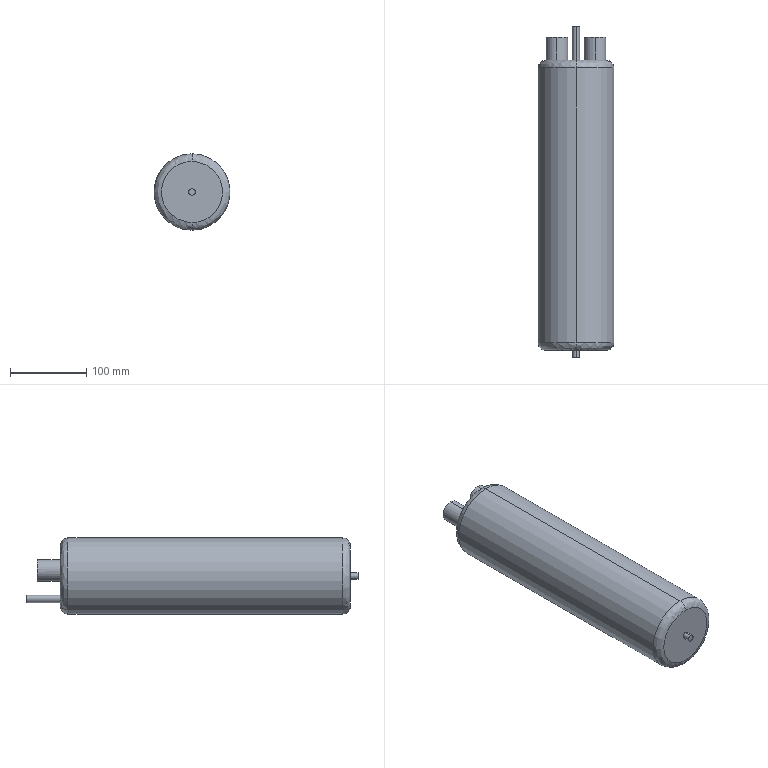Part | STEP file | PN_0001-1-1-8-oil separator 28 | 1 solid | 31 faces | box 100 x 435 x 100 mm | volume 2983083 mm3 | cylinder 16 | plane 11 | spline 4 | commonest cylinder face diameters 24 x4 28 x4 8 x2 8.5 x2 9.6 x2 100 x2